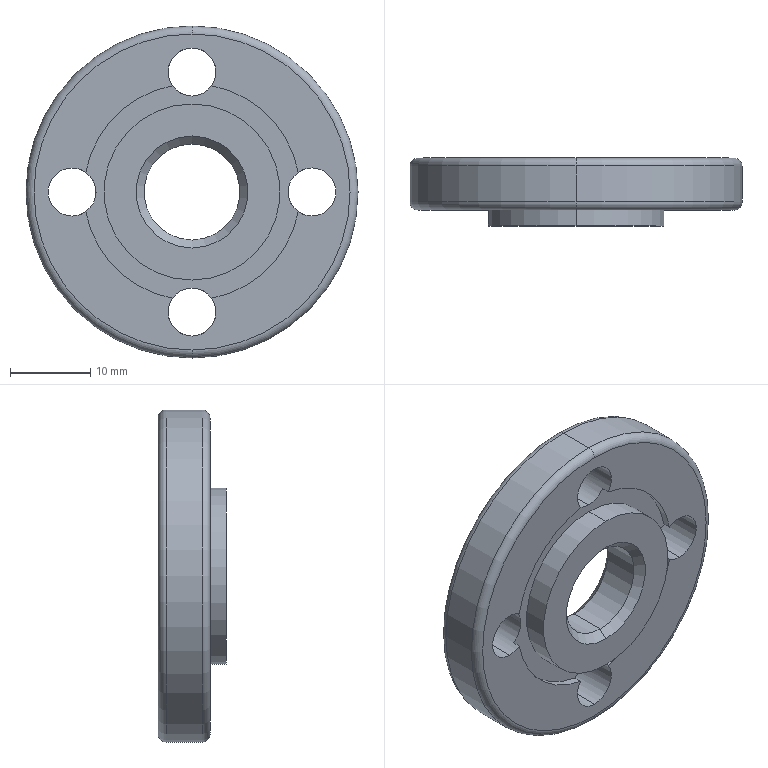Part | SolidWorks | features BaseBody 1 | 1 solid | 33 faces | box 41.5 x 8.5 x 41.5 mm | volume 6920 mm3 | cylinder 18 | cone 6 | plane 5 | torus 4 | commonest cylinder face diameters 6 x8 27 x4 12 x2 22 x2 41.5 x2
STEP:
#1=CARTESIAN_POINT('',(-15.,2.,3.));
#2=VERTEX_POINT('',#1);
#3=CARTESIAN_POINT('',(-15.,2.,-3.));
#4=VERTEX_POINT('',#3);
#5=CARTESIAN_POINT('',(-15.,2.,0.));
#6=DIRECTION('',(0.,-1.,0.));
#7=DIRECTION('',(0.,0.,-1.));
#8=AXIS2_PLACEMENT_3D('',#5,#6,#7);
#9=CIRCLE('',#8,3.);
#10=EDGE_CURVE('',#2,#4,#9,.T.);
#11=ORIENTED_EDGE('',*,*,#10,.T.);
#12=CARTESIAN_POINT('',(-15.,8.5,-3.));
#13=VERTEX_POINT('',#12);
#14=CARTESIAN_POINT('',(-15.,-1.5,-3.));
#15=DIRECTION('',(0.,1.,0.));
#16=VECTOR('',#15,1000.);
#17=LINE('',#14,#16);
#18=EDGE_CURVE('',#4,#13,#17,.T.);
#19=ORIENTED_EDGE('',*,*,#18,.T.);
#20=CARTESIAN_POINT('',(-15.,8.5,3.));
#21=VERTEX_POINT('',#20);
#22=CARTESIAN_POINT('',(-15.,8.5,0.));
#23=DIRECTION('',(0.,1.,0.));
#24=DIRECTION('',(1.,0.,0.));
#25=AXIS2_PLACEMENT_3D('',#22,#23,#24);
#26=CIRCLE('',#25,3.);
#27=EDGE_CURVE('',#13,#21,#26,.T.);
#28=ORIENTED_EDGE('',*,*,#27,.T.);
#29=CARTESIAN_POINT('',(-15.,-1.5,3.));
#30=DIRECTION('',(0.,1.,0.));
#31=VECTOR('',#30,1000.);
#32=LINE('',#29,#31);
#33=EDGE_CURVE('',#2,#21,#32,.T.);
#34=ORIENTED_EDGE('',*,*,#33,.F.);
#35=EDGE_LOOP('',(#11,#19,#28,#34));
#36=FACE_OUTER_BOUND('',#35,.T.);
#37=CARTESIAN_POINT('',(-15.,-1.5,0.));
#38=DIRECTION('',(0.,1.,0.));
#39=DIRECTION('',(0.,0.,1.));
#40=AXIS2_PLACEMENT_3D('',#37,#38,#39);
#41=CYLINDRICAL_SURFACE('',#40,3.);
#42=ADVANCED_FACE('',(#36),#41,.F.);
#43=CARTESIAN_POINT('',(-2.454,3.,13.275));
#44=VERTEX_POINT('',#43);
#45=CARTESIAN_POINT('',(0.,3.,12.));
#46=VERTEX_POINT('',#45);
#47=CARTESIAN_POINT('',(0.,3.,15.));
#48=DIRECTION('',(0.,-1.,0.));
#49=DIRECTION('',(0.,0.,-1.));
#50=AXIS2_PLACEMENT_3D('',#47,#48,#49);
#51=CIRCLE('',#50,3.);
#52=EDGE_CURVE('',#44,#46,#51,.T.);
#53=ORIENTED_EDGE('',*,*,#52,.T.);
#54=CARTESIAN_POINT('',(0.,7.35,12.));
#55=VERTEX_POINT('',#54);
#56=CARTESIAN_POINT('',(0.,-1.5,12.));
#57=DIRECTION('',(0.,1.,0.));
#58=VECTOR('',#57,1000.);
#59=LINE('',#56,#58);
#60=EDGE_CURVE('',#46,#55,#59,.T.);
#61=ORIENTED_EDGE('',*,*,#60,.T.);
#62=CARTESIAN_POINT('',(-2.203,8.5,12.964));
#63=VERTEX_POINT('',#62);
#64=CARTESIAN_POINT('',(0.,7.35,12.));
#65=CARTESIAN_POINT('',(-0.2354,7.35,12.));
#66=CARTESIAN_POINT('',(-0.4621,7.384,12.027));
#67=CARTESIAN_POINT('',(-0.9003,7.511,12.129));
#68=CARTESIAN_POINT('',(-1.104,7.601,12.203));
#69=CARTESIAN_POINT('',(-1.477,7.817,12.381));
#70=CARTESIAN_POINT('',(-1.646,7.942,12.485));
#71=CARTESIAN_POINT('',(-1.947,8.208,12.71));
#72=CARTESIAN_POINT('',(-2.082,8.35,12.833));
#73=CARTESIAN_POINT('',(-2.203,8.5,12.964));
#74=B_SPLINE_CURVE_WITH_KNOTS('',3,(#64,#65,#66,#67,#68,#69,#70,#71,#72,#73),.UNSPECIFIED.,.F.,.F.,(4,2,2,2,4),(0.,0.0006925,0.001385,0.002078,0.00277),.UNSPECIFIED.);
#75=EDGE_CURVE('',#55,#63,#74,.T.);
#76=ORIENTED_EDGE('',*,*,#75,.T.);
#77=CARTESIAN_POINT('',(0.,8.5,18.));
#78=VERTEX_POINT('',#77);
#79=CARTESIAN_POINT('',(0.,8.5,15.));
#80=DIRECTION('',(0.,1.,0.));
#81=DIRECTION('',(0.,0.,-1.));
#82=AXIS2_PLACEMENT_3D('',#79,#80,#81);
#83=CIRCLE('',#82,3.);
#84=EDGE_CURVE('',#63,#78,#83,.T.);
#85=ORIENTED_EDGE('',*,*,#84,.T.);
#86=CARTESIAN_POINT('',(0.,2.,18.));
#87=VERTEX_POINT('',#86);
#88=CARTESIAN_POINT('',(0.,-1.5,18.));
#89=DIRECTION('',(0.,1.,0.));
#90=VECTOR('',#89,1000.);
#91=LINE('',#88,#90);
#92=EDGE_CURVE('',#87,#78,#91,.T.);
#93=ORIENTED_EDGE('',*,*,#92,.F.);
#94=CARTESIAN_POINT('',(-2.454,2.,13.275));
#95=VERTEX_POINT('',#94);
#96=CARTESIAN_POINT('',(0.,2.,15.));
#97=DIRECTION('',(0.,-1.,0.));
#98=DIRECTION('',(0.,0.,-1.));
#99=AXIS2_PLACEMENT_3D('',#96,#97,#98);
#100=CIRCLE('',#99,3.);
#101=EDGE_CURVE('',#87,#95,#100,.T.);
#102=ORIENTED_EDGE('',*,*,#101,.T.);
#103=CARTESIAN_POINT('',(-2.454,3.5,13.275));
#104=DIRECTION('',(0.,1.,0.));
#105=VECTOR('',#104,1000.);
#106=LINE('',#103,#105);
#107=EDGE_CURVE('',#95,#44,#106,.T.);
#108=ORIENTED_EDGE('',*,*,#107,.T.);
#109=EDGE_LOOP('',(#53,#61,#76,#85,#93,#102,#108));
#110=FACE_OUTER_BOUND('',#109,.T.);
#111=CARTESIAN_POINT('',(0.,-1.5,15.));
#112=DIRECTION('',(0.,1.,0.));
#113=DIRECTION('',(0.,0.,1.));
#114=AXIS2_PLACEMENT_3D('',#111,#112,#113);
#115=CYLINDRICAL_SURFACE('',#114,3.);
#116=ADVANCED_FACE('',(#110),#115,.F.);
#117=CARTESIAN_POINT('',(13.275,2.,-2.454));
#118=VERTEX_POINT('',#117);
#119=CARTESIAN_POINT('',(15.,2.,-3.));
#120=VERTEX_POINT('',#119);
#121=CARTESIAN_POINT('',(15.,2.,0.));
#122=DIRECTION('',(0.,-1.,0.));
#123=DIRECTION('',(0.,0.,-1.));
#124=AXIS2_PLACEMENT_3D('',#121,#122,#123);
#125=CIRCLE('',#124,3.);
#126=EDGE_CURVE('',#118,#120,#125,.T.);
#127=ORIENTED_EDGE('',*,*,#126,.T.);
#128=CARTESIAN_POINT('',(15.,8.5,-3.));
#129=VERTEX_POINT('',#128);
#130=CARTESIAN_POINT('',(15.,-1.5,-3.));
#131=DIRECTION('',(0.,1.,0.));
#132=VECTOR('',#131,1000.);
#133=LINE('',#130,#132);
#134=EDGE_CURVE('',#120,#129,#133,.T.);
#135=ORIENTED_EDGE('',*,*,#134,.T.);
#136=CARTESIAN_POINT('',(12.964,8.5,-2.203));
#137=VERTEX_POINT('',#136);
#138=CARTESIAN_POINT('',(15.,8.5,0.));
#139=DIRECTION('',(0.,1.,0.));
#140=DIRECTION('',(-1.,0.,0.));
#141=AXIS2_PLACEMENT_3D('',#138,#139,#140);
#142=CIRCLE('',#141,3.);
#143=EDGE_CURVE('',#129,#137,#142,.T.);
#144=ORIENTED_EDGE('',*,*,#143,.T.);
#145=CARTESIAN_POINT('',(12.964,8.5,2.203));
#146=VERTEX_POINT('',#145);
#147=CARTESIAN_POINT('',(12.964,8.5,-2.203));
#148=CARTESIAN_POINT('',(12.833,8.35,-2.082));
#149=CARTESIAN_POINT('',(12.71,8.208,-1.948));
#150=CARTESIAN_POINT('',(12.485,7.942,-1.646));
#151=CARTESIAN_POINT('',(12.38,7.817,-1.477));
#152=CARTESIAN_POINT('',(12.203,7.602,-1.105));
#153=CARTESIAN_POINT('',(12.13,7.512,-0.9023));
#154=CARTESIAN_POINT('',(12.053,7.417,-0.5748));
#155=CARTESIAN_POINT('',(12.034,7.392,-0.4634));
#156=CARTESIAN_POINT('',(12.007,7.359,-0.2357));
#157=CARTESIAN_POINT('',(12.,7.35,-0.1181));
#158=CARTESIAN_POINT('',(12.,7.35,0.1144));
#159=CARTESIAN_POINT('',(12.007,7.358,0.2295));
#160=CARTESIAN_POINT('',(12.033,7.391,0.4574));
#161=CARTESIAN_POINT('',(12.053,7.416,0.5711));
#162=CARTESIAN_POINT('',(12.129,7.51,0.8984));
#163=CARTESIAN_POINT('',(12.203,7.601,1.103));
#164=CARTESIAN_POINT('',(12.468,7.923,1.66));
#165=CARTESIAN_POINT('',(12.701,8.2,1.961));
#166=CARTESIAN_POINT('',(12.964,8.5,2.203));
#167=B_SPLINE_CURVE_WITH_KNOTS('',3,(#147,#148,#149,#150,#151,#152,#153,#154,#155,#156,#157,#158,#159,#160,#161,#162,#163,#164,#165,#166),.UNSPECIFIED.,.F.,.F.,(4,2,2,2,2,2,2,2,2,4),(0.,0.0006916,0.001383,0.002075,0.00242,0.002766,0.003112,0.003458,0.004149,0.005533),.UNSPECIFIED.);
#168=EDGE_CURVE('',#137,#146,#167,.T.);
#169=ORIENTED_EDGE('',*,*,#168,.T.);
#170=CARTESIAN_POINT('',(15.,8.5,3.));
#171=VERTEX_POINT('',#170);
#172=CARTESIAN_POINT('',(15.,8.5,0.));
#173=DIRECTION('',(0.,1.,0.));
#174=DIRECTION('',(-1.,0.,0.));
#175=AXIS2_PLACEMENT_3D('',#172,#173,#174);
#176=CIRCLE('',#175,3.);
#177=EDGE_CURVE('',#146,#171,#176,.T.);
#178=ORIENTED_EDGE('',*,*,#177,.T.);
#179=CARTESIAN_POINT('',(15.,2.,3.));
#180=VERTEX_POINT('',#179);
#181=CARTESIAN_POINT('',(15.,-1.5,3.));
#182=DIRECTION('',(0.,1.,0.));
#183=VECTOR('',#182,1000.);
#184=LINE('',#181,#183);
#185=EDGE_CURVE('',#180,#171,#184,.T.);
#186=ORIENTED_EDGE('',*,*,#185,.F.);
#187=CARTESIAN_POINT('',(13.275,2.,2.454));
#188=VERTEX_POINT('',#187);
#189=CARTESIAN_POINT('',(15.,2.,0.));
#190=DIRECTION('',(0.,-1.,0.));
#191=DIRECTION('',(0.,0.,-1.));
#192=AXIS2_PLACEMENT_3D('',#189,#190,#191);
#193=CIRCLE('',#192,3.);
#194=EDGE_CURVE('',#180,#188,#193,.T.);
#195=ORIENTED_EDGE('',*,*,#194,.T.);
#196=CARTESIAN_POINT('',(13.275,3.,2.454));
#197=VERTEX_POINT('',#196);
#198=CARTESIAN_POINT('',(13.275,3.5,2.454));
#199=DIRECTION('',(0.,1.,0.));
#200=VECTOR('',#199,1000.);
#201=LINE('',#198,#200);
#202=EDGE_CURVE('',#188,#197,#201,.T.);
#203=ORIENTED_EDGE('',*,*,#202,.T.);
#204=CARTESIAN_POINT('',(13.275,3.,-2.454));
#205=VERTEX_POINT('',#204);
#206=CARTESIAN_POINT('',(15.,3.,0.));
#207=DIRECTION('',(0.,-1.,0.));
#208=DIRECTION('',(0.,0.,-1.));
#209=AXIS2_PLACEMENT_3D('',#206,#207,#208);
#210=CIRCLE('',#209,3.);
#211=EDGE_CURVE('',#197,#205,#210,.T.);
#212=ORIENTED_EDGE('',*,*,#211,.T.);
#213=CARTESIAN_POINT('',(13.275,3.5,-2.454));
#214=DIRECTION('',(0.,-1.,0.));
#215=VECTOR('',#214,1000.);
#216=LINE('',#213,#215);
#217=EDGE_CURVE('',#205,#118,#216,.T.);
#218=ORIENTED_EDGE('',*,*,#217,.T.);
#219=EDGE_LOOP('',(#127,#135,#144,#169,#178,#186,#195,#203,#212,#218));
#220=FACE_OUTER_BOUND('',#219,.T.);
#221=CARTESIAN_POINT('',(15.,-1.5,0.));
#222=DIRECTION('',(0.,1.,0.));
#223=DIRECTION('',(0.,0.,1.));
#224=AXIS2_PLACEMENT_3D('',#221,#222,#223);
#225=CYLINDRICAL_SURFACE('',#224,3.);
#226=ADVANCED_FACE('',(#220),#225,.F.);
#227=CARTESIAN_POINT('',(-2.454,2.,-13.275));
#228=VERTEX_POINT('',#227);
#229=CARTESIAN_POINT('',(0.,2.,-18.));
#230=VERTEX_POINT('',#229);
#231=CARTESIAN_POINT('',(0.,2.,-15.));
#232=DIRECTION('',(0.,-1.,0.));
#233=DIRECTION('',(0.,0.,-1.));
#234=AXIS2_PLACEMENT_3D('',#231,#232,#233);
#235=CIRCLE('',#234,3.);
#236=EDGE_CURVE('',#228,#230,#235,.T.);
#237=ORIENTED_EDGE('',*,*,#236,.T.);
#238=CARTESIAN_POINT('',(0.,8.5,-18.));
#239=VERTEX_POINT('',#238);
#240=CARTESIAN_POINT('',(0.,-1.5,-18.));
#241=DIRECTION('',(0.,1.,0.));
#242=VECTOR('',#241,1000.);
#243=LINE('',#240,#242);
#244=EDGE_CURVE('',#230,#239,#243,.T.);
#245=ORIENTED_EDGE('',*,*,#244,.T.);
#246=CARTESIAN_POINT('',(-2.203,8.5,-12.964));
#247=VERTEX_POINT('',#246);
#248=CARTESIAN_POINT('',(0.,8.5,-15.));
#249=DIRECTION('',(0.,1.,0.));
#250=DIRECTION('',(0.,0.,1.));
#251=AXIS2_PLACEMENT_3D('',#248,#249,#250);
#252=CIRCLE('',#251,3.);
#253=EDGE_CURVE('',#239,#247,#252,.T.);
#254=ORIENTED_EDGE('',*,*,#253,.T.);
#255=CARTESIAN_POINT('',(0.,7.35,-12.));
#256=VERTEX_POINT('',#255);
#257=CARTESIAN_POINT('',(-2.203,8.5,-12.964));
#258=CARTESIAN_POINT('',(-2.082,8.35,-12.833));
#259=CARTESIAN_POINT('',(-1.947,8.208,-12.71));
#260=CARTESIAN_POINT('',(-1.646,7.942,-12.485));
#261=CARTESIAN_POINT('',(-1.476,7.817,-12.38));
#262=CARTESIAN_POINT('',(-1.105,7.602,-12.203));
#263=CARTESIAN_POINT('',(-0.9015,7.511,-12.13));
#264=CARTESIAN_POINT('',(-0.4646,7.385,-12.028));
#265=CARTESIAN_POINT('',(-0.2349,7.35,-12.));
#266=CARTESIAN_POINT('',(0.,7.35,-12.));
#267=B_SPLINE_CURVE_WITH_KNOTS('',3,(#257,#258,#259,#260,#261,#262,#263,#264,#265,#266),.UNSPECIFIED.,.F.,.F.,(4,2,2,2,4),(0.,0.0006919,0.001384,0.002076,0.002768),.UNSPECIFIED.);
#268=EDGE_CURVE('',#247,#256,#267,.T.);
#269=ORIENTED_EDGE('',*,*,#268,.T.);
#270=CARTESIAN_POINT('',(0.,3.,-12.));
#271=VERTEX_POINT('',#270);
#272=CARTESIAN_POINT('',(0.,-1.5,-12.));
#273=DIRECTION('',(0.,1.,0.));
#274=VECTOR('',#273,1000.);
#275=LINE('',#272,#274);
#276=EDGE_CURVE('',#271,#256,#275,.T.);
#277=ORIENTED_EDGE('',*,*,#276,.F.);
#278=CARTESIAN_POINT('',(-2.454,3.,-13.275));
#279=VERTEX_POINT('',#278);
#280=CARTESIAN_POINT('',(0.,3.,-15.));
#281=DIRECTION('',(0.,-1.,0.));
#282=DIRECTION('',(0.,0.,-1.));
#283=AXIS2_PLACEMENT_3D('',#280,#281,#282);
#284=CIRCLE('',#283,3.);
#285=EDGE_CURVE('',#271,#279,#284,.T.);
#286=ORIENTED_EDGE('',*,*,#285,.T.);
#287=CARTESIAN_POINT('',(-2.454,3.5,-13.275));
#288=DIRECTION('',(0.,-1.,0.));
#289=VECTOR('',#288,1000.);
#290=LINE('',#287,#289);
#291=EDGE_CURVE('',#279,#228,#290,.T.);
#292=ORIENTED_EDGE('',*,*,#291,.T.);
#293=EDGE_LOOP('',(#237,#245,#254,#269,#277,#286,#292));
#294=FACE_OUTER_BOUND('',#293,.T.);
#295=CARTESIAN_POINT('',(0.,-1.5,-15.));
#296=DIRECTION('',(0.,1.,0.));
#297=DIRECTION('',(0.,0.,1.));
#298=AXIS2_PLACEMENT_3D('',#295,#296,#297);
#299=CYLINDRICAL_SURFACE('',#298,3.);
#300=ADVANCED_FACE('',(#294),#299,.F.);
#301=CARTESIAN_POINT('',(0.,6.6,11.25));
#302=VERTEX_POINT('',#301);
#303=CARTESIAN_POINT('',(0.,6.6,-11.25));
#304=VERTEX_POINT('',#303);
#305=CARTESIAN_POINT('',(0.,6.6,0.));
#306=DIRECTION('',(0.,-1.,0.));
#307=DIRECTION('',(0.,0.,-1.));
#308=AXIS2_PLACEMENT_3D('',#305,#306,#307);
#309=CIRCLE('',#308,11.25);
#310=EDGE_CURVE('',#302,#304,#309,.T.);
#311=ORIENTED_EDGE('',*,*,#310,.T.);
#312=CARTESIAN_POINT('',(0.,8.5,-13.15));
#313=DIRECTION('',(0.,0.7071,-0.7071));
#314=VECTOR('',#313,1000.);
#315=LINE('',#312,#314);
#316=EDGE_CURVE('',#304,#256,#315,.T.);
#317=ORIENTED_EDGE('',*,*,#316,.T.);
#318=ORIENTED_EDGE('',*,*,#268,.F.);
#319=CARTESIAN_POINT('',(-12.964,8.5,-2.203));
#320=VERTEX_POINT('',#319);
#321=CARTESIAN_POINT('',(0.,8.5,0.));
#322=DIRECTION('',(0.,-1.,0.));
#323=DIRECTION('',(0.,0.,1.));
#324=AXIS2_PLACEMENT_3D('',#321,#322,#323);
#325=CIRCLE('',#324,13.15);
#326=EDGE_CURVE('',#320,#247,#325,.T.);
#327=ORIENTED_EDGE('',*,*,#326,.F.);
#328=CARTESIAN_POINT('',(-12.964,8.5,2.203));
#329=VERTEX_POINT('',#328);
#330=CARTESIAN_POINT('',(-12.964,8.5,2.203));
#331=CARTESIAN_POINT('',(-12.833,8.35,2.082));
#332=CARTESIAN_POINT('',(-12.71,8.208,1.948));
#333=CARTESIAN_POINT('',(-12.485,7.942,1.646));
#334=CARTESIAN_POINT('',(-12.38,7.817,1.477));
#335=CARTESIAN_POINT('',(-12.203,7.602,1.105));
#336=CARTESIAN_POINT('',(-12.13,7.512,0.9023));
#337=CARTESIAN_POINT('',(-12.053,7.417,0.5748));
#338=CARTESIAN_POINT('',(-12.034,7.392,0.4634));
#339=CARTESIAN_POINT('',(-12.007,7.359,0.2357));
#340=CARTESIAN_POINT('',(-12.,7.35,0.1181));
#341=CARTESIAN_POINT('',(-12.,7.35,-0.1144));
#342=CARTESIAN_POINT('',(-12.007,7.358,-0.2295));
#343=CARTESIAN_POINT('',(-12.033,7.391,-0.4574));
#344=CARTESIAN_POINT('',(-12.053,7.416,-0.5711));
#345=CARTESIAN_POINT('',(-12.129,7.51,-0.8984));
#346=CARTESIAN_POINT('',(-12.203,7.601,-1.103));
#347=CARTESIAN_POINT('',(-12.468,7.923,-1.66));
#348=CARTESIAN_POINT('',(-12.701,8.2,-1.961));
#349=CARTESIAN_POINT('',(-12.964,8.5,-2.203));
#350=B_SPLINE_CURVE_WITH_KNOTS('',3,(#330,#331,#332,#333,#334,#335,#336,#337,#338,#339,#340,#341,#342,#343,#344,#345,#346,#347,#348,#349),.UNSPECIFIED.,.F.,.F.,(4,2,2,2,2,2,2,2,2,4),(0.,0.0006916,0.001383,0.002075,0.00242,0.002766,0.003112,0.003458,0.004149,0.005533),.UNSPECIFIED.);
#351=EDGE_CURVE('',#329,#320,#350,.T.);
#352=ORIENTED_EDGE('',*,*,#351,.F.);
#353=CARTESIAN_POINT('',(0.,8.5,0.));
#354=DIRECTION('',(0.,-1.,0.));
#355=DIRECTION('',(0.,0.,1.));
#356=AXIS2_PLACEMENT_3D('',#353,#354,#355);
#357=CIRCLE('',#356,13.15);
#358=EDGE_CURVE('',#63,#329,#357,.T.);
#359=ORIENTED_EDGE('',*,*,#358,.F.);
#360=ORIENTED_EDGE('',*,*,#75,.F.);
#361=CARTESIAN_POINT('',(0.,8.5,13.15));
#362=DIRECTION('',(0.,0.7071,0.7071));
#363=VECTOR('',#362,1000.);
#364=LINE('',#361,#363);
#365=EDGE_CURVE('',#302,#55,#364,.T.);
#366=ORIENTED_EDGE('',*,*,#365,.F.);
#367=EDGE_LOOP('',(#311,#317,#318,#327,#352,#359,#360,#366));
#368=FACE_OUTER_BOUND('',#367,.T.);
#369=CARTESIAN_POINT('',(0.,8.5,0.));
#370=DIRECTION('',(0.,1.,0.));
#371=DIRECTION('',(0.,0.,1.));
#372=AXIS2_PLACEMENT_3D('',#369,#370,#371);
#373=CONICAL_SURFACE('',#372,13.15,0.7854);
#374=ADVANCED_FACE('',(#368),#373,.F.);
#375=CARTESIAN_POINT('',(0.,7.5,-20.75));
#376=VERTEX_POINT('',#375);
#377=CARTESIAN_POINT('',(0.,7.5,20.75));
#378=VERTEX_POINT('',#377);
#379=CARTESIAN_POINT('',(0.,7.5,0.));
#380=DIRECTION('',(0.,-1.,0.));
#381=DIRECTION('',(0.,0.,1.));
#382=AXIS2_PLACEMENT_3D('',#379,#380,#381);
#383=CIRCLE('',#382,20.75);
#384=EDGE_CURVE('',#376,#378,#383,.T.);
#385=ORIENTED_EDGE('',*,*,#384,.F.);
#386=CARTESIAN_POINT('',(0.,8.5,-19.75));
#387=VERTEX_POINT('',#386);
#388=CARTESIAN_POINT('',(0.,7.5,-19.75));
#389=DIRECTION('',(1.,0.,0.));
#390=DIRECTION('',(0.,0.,-1.));
#391=AXIS2_PLACEMENT_3D('',#388,#389,#390);
#392=CIRCLE('',#391,1.);
#393=EDGE_CURVE('',#376,#387,#392,.T.);
#394=ORIENTED_EDGE('',*,*,#393,.T.);
#395=CARTESIAN_POINT('',(0.,8.5,19.75));
#396=VERTEX_POINT('',#395);
#397=CARTESIAN_POINT('',(0.,8.5,0.));
#398=DIRECTION('',(0.,1.,0.));
#399=DIRECTION('',(0.,0.,1.));
#400=AXIS2_PLACEMENT_3D('',#397,#398,#399);
#401=CIRCLE('',#400,19.75);
#402=EDGE_CURVE('',#396,#387,#401,.T.);
#403=ORIENTED_EDGE('',*,*,#402,.F.);
#404=CARTESIAN_POINT('',(0.,7.5,19.75));
#405=DIRECTION('',(-1.,0.,0.));
#406=DIRECTION('',(0.,0.,1.));
#407=AXIS2_PLACEMENT_3D('',#404,#405,#406);
#408=CIRCLE('',#407,1.);
#409=EDGE_CURVE('',#378,#396,#408,.T.);
#410=ORIENTED_EDGE('',*,*,#409,.F.);
#411=EDGE_LOOP('',(#385,#394,#403,#410));
#412=FACE_OUTER_BOUND('',#411,.T.);
#413=CARTESIAN_POINT('',(0.,7.5,0.));
#414=DIRECTION('',(0.,1.,0.));
#415=DIRECTION('',(0.,0.,1.));
#416=AXIS2_PLACEMENT_3D('',#413,#414,#415);
#417=TOROIDAL_SURFACE('',#416,19.75,1.);
#418=ADVANCED_FACE('',(#412),#417,.T.);
#419=CARTESIAN_POINT('',(0.,3.,20.75));
#420=VERTEX_POINT('',#419);
#421=CARTESIAN_POINT('',(0.,3.,-20.75));
#422=VERTEX_POINT('',#421);
#423=CARTESIAN_POINT('',(0.,3.,0.));
#424=DIRECTION('',(0.,1.,0.));
#425=DIRECTION('',(0.,0.,-1.));
#426=AXIS2_PLACEMENT_3D('',#423,#424,#425);
#427=CIRCLE('',#426,20.75);
#428=EDGE_CURVE('',#420,#422,#427,.T.);
#429=ORIENTED_EDGE('',*,*,#428,.F.);
#430=CARTESIAN_POINT('',(0.,2.,19.75));
#431=VERTEX_POINT('',#430);
#432=CARTESIAN_POINT('',(0.,3.,19.75));
#433=DIRECTION('',(1.,0.,0.));
#434=DIRECTION('',(0.,0.,-1.));
#435=AXIS2_PLACEMENT_3D('',#432,#433,#434);
#436=CIRCLE('',#435,1.);
#437=EDGE_CURVE('',#420,#431,#436,.T.);
#438=ORIENTED_EDGE('',*,*,#437,.T.);
#439=CARTESIAN_POINT('',(0.,2.,-19.75));
#440=VERTEX_POINT('',#439);
#441=CARTESIAN_POINT('',(0.,2.,0.));
#442=DIRECTION('',(0.,-1.,0.));
#443=DIRECTION('',(0.,0.,-1.));
#444=AXIS2_PLACEMENT_3D('',#441,#442,#443);
#445=CIRCLE('',#444,19.75);
#446=EDGE_CURVE('',#440,#431,#445,.T.);
#447=ORIENTED_EDGE('',*,*,#446,.F.);
#448=CARTESIAN_POINT('',(0.,3.,-19.75));
#449=DIRECTION('',(-1.,0.,0.));
#450=DIRECTION('',(0.,0.,1.));
#451=AXIS2_PLACEMENT_3D('',#448,#449,#450);
#452=CIRCLE('',#451,1.);
#453=EDGE_CURVE('',#422,#440,#452,.T.);
#454=ORIENTED_EDGE('',*,*,#453,.F.);
#455=EDGE_LOOP('',(#429,#438,#447,#454));
#456=FACE_OUTER_BOUND('',#455,.T.);
#457=CARTESIAN_POINT('',(0.,3.,0.));
#458=DIRECTION('',(0.,-1.,0.));
#459=DIRECTION('',(0.,0.,-1.));
#460=AXIS2_PLACEMENT_3D('',#457,#458,#459);
#461=TOROIDAL_SURFACE('',#460,19.75,1.);
#462=ADVANCED_FACE('',(#456),#461,.T.);
#463=CARTESIAN_POINT('',(0.,1.,6.));
#464=VERTEX_POINT('',#463);
#465=CARTESIAN_POINT('',(0.,1.,-6.));
#466=VERTEX_POINT('',#465);
#467=CARTESIAN_POINT('',(0.,1.,0.));
#468=DIRECTION('',(0.,-1.,0.));
#469=DIRECTION('',(0.,0.,-1.));
#470=AXIS2_PLACEMENT_3D('',#467,#468,#469);
#471=CIRCLE('',#470,6.);
#472=EDGE_CURVE('',#464,#466,#471,.T.);
#473=ORIENTED_EDGE('',*,*,#472,.F.);
#474=CARTESIAN_POINT('',(0.,0.,7.));
#475=VERTEX_POINT('',#474);
#476=CARTESIAN_POINT('',(0.,1.,6.));
#477=DIRECTION('',(0.,-0.7071,0.7071));
#478=VECTOR('',#477,1000.);
#479=LINE('',#476,#478);
#480=EDGE_CURVE('',#464,#475,#479,.T.);
#481=ORIENTED_EDGE('',*,*,#480,.T.);
#482=CARTESIAN_POINT('',(0.,0.,-7.));
#483=VERTEX_POINT('',#482);
#484=CARTESIAN_POINT('',(0.,0.,0.));
#485=DIRECTION('',(0.,1.,0.));
#486=DIRECTION('',(0.,0.,-1.));
#487=AXIS2_PLACEMENT_3D('',#484,#485,#486);
#488=CIRCLE('',#487,7.);
#489=EDGE_CURVE('',#483,#475,#488,.T.);
#490=ORIENTED_EDGE('',*,*,#489,.F.);
#491=CARTESIAN_POINT('',(0.,1.,-6.));
#492=DIRECTION('',(0.,-0.7071,-0.7071));
#493=VECTOR('',#492,1000.);
#494=LINE('',#491,#493);
#495=EDGE_CURVE('',#466,#483,#494,.T.);
#496=ORIENTED_EDGE('',*,*,#495,.F.);
#497=EDGE_LOOP('',(#473,#481,#490,#496));
#498=FACE_OUTER_BOUND('',#497,.T.);
#499=CARTESIAN_POINT('',(0.,1.,0.));
#500=DIRECTION('',(0.,-1.,0.));
#501=DIRECTION('',(0.,0.,-1.));
#502=AXIS2_PLACEMENT_3D('',#499,#500,#501);
#503=CONICAL_SURFACE('',#502,6.,0.7854);
#504=ADVANCED_FACE('',(#498),#503,.F.);
#505=CARTESIAN_POINT('',(0.,5.6,-6.));
#506=VERTEX_POINT('',#505);
#507=CARTESIAN_POINT('',(0.,5.6,6.));
#508=VERTEX_POINT('',#507);
#509=CARTESIAN_POINT('',(0.,5.6,0.));
#510=DIRECTION('',(0.,1.,0.));
#511=DIRECTION('',(0.,0.,1.));
#512=AXIS2_PLACEMENT_3D('',#509,#510,#511);
#513=CIRCLE('',#512,6.);
#514=EDGE_CURVE('',#506,#508,#513,.T.);
#515=ORIENTED_EDGE('',*,*,#514,.F.);
#516=CARTESIAN_POINT('',(0.,6.6,-7.));
#517=VERTEX_POINT('',#516);
#518=CARTESIAN_POINT('',(0.,6.6,-7.));
#519=DIRECTION('',(0.,0.7071,-0.7071));
#520=VECTOR('',#519,1000.);
#521=LINE('',#518,#520);
#522=EDGE_CURVE('',#506,#517,#521,.T.);
#523=ORIENTED_EDGE('',*,*,#522,.T.);
#524=CARTESIAN_POINT('',(0.,6.6,7.));
#525=VERTEX_POINT('',#524);
#526=CARTESIAN_POINT('',(0.,6.6,0.));
#527=DIRECTION('',(0.,-1.,0.));
#528=DIRECTION('',(0.,0.,1.));
#529=AXIS2_PLACEMENT_3D('',#526,#527,#528);
#530=CIRCLE('',#529,7.);
#531=EDGE_CURVE('',#525,#517,#530,.T.);
#532=ORIENTED_EDGE('',*,*,#531,.F.);
#533=CARTESIAN_POINT('',(0.,6.6,7.));
#534=DIRECTION('',(0.,0.7071,0.7071));
#535=VECTOR('',#534,1000.);
#536=LINE('',#533,#535);
#537=EDGE_CURVE('',#508,#525,#536,.T.);
#538=ORIENTED_EDGE('',*,*,#537,.F.);
#539=EDGE_LOOP('',(#515,#523,#532,#538));
#540=FACE_OUTER_BOUND('',#539,.T.);
#541=CARTESIAN_POINT('',(0.,6.6,0.));
#542=DIRECTION('',(0.,1.,0.));
#543=DIRECTION('',(0.,0.,1.));
#544=AXIS2_PLACEMENT_3D('',#541,#542,#543);
#545=CONICAL_SURFACE('',#544,7.,0.7854);
#546=ADVANCED_FACE('',(#540),#545,.F.);
#547=ORIENTED_EDGE('',*,*,#384,.T.);
#548=CARTESIAN_POINT('',(0.,0.,20.75));
#549=DIRECTION('',(0.,-1.,0.));
#550=VECTOR('',#549,1000.);
#551=LINE('',#548,#550);
#552=EDGE_CURVE('',#378,#420,#551,.T.);
#553=ORIENTED_EDGE('',*,*,#552,.T.);
#554=ORIENTED_EDGE('',*,*,#428,.T.);
#555=CARTESIAN_POINT('',(0.,0.,-20.75));
#556=DIRECTION('',(0.,-1.,0.));
#557=VECTOR('',#556,1000.);
#558=LINE('',#555,#557);
#559=EDGE_CURVE('',#376,#422,#558,.T.);
#560=ORIENTED_EDGE('',*,*,#559,.F.);
#561=EDGE_LOOP('',(#547,#553,#554,#560));
#562=FACE_OUTER_BOUND('',#561,.T.);
#563=CARTESIAN_POINT('',(0.,0.,0.));
#564=DIRECTION('',(0.,-1.,0.));
#565=DIRECTION('',(0.,0.,-1.));
#566=AXIS2_PLACEMENT_3D('',#563,#564,#565);
#567=CYLINDRICAL_SURFACE('',#566,20.75);
#568=ADVANCED_FACE('',(#562),#567,.T.);
#569=CARTESIAN_POINT('',(0.,3.,-11.));
#570=VERTEX_POINT('',#569);
#571=CARTESIAN_POINT('',(0.,3.,11.));
#572=VERTEX_POINT('',#571);
#573=CARTESIAN_POINT('',(0.,3.,0.));
#574=DIRECTION('',(0.,-1.,0.));
#575=DIRECTION('',(0.,0.,-1.));
#576=AXIS2_PLACEMENT_3D('',#573,#574,#575);
#577=CIRCLE('',#576,11.);
#578=EDGE_CURVE('',#570,#572,#577,.T.);
#579=ORIENTED_EDGE('',*,*,#578,.T.);
#580=CARTESIAN_POINT('',(0.,0.,11.));
#581=VERTEX_POINT('',#580);
#582=CARTESIAN_POINT('',(0.,0.,11.));
#583=DIRECTION('',(0.,-1.,0.));
#584=VECTOR('',#583,1000.);
#585=LINE('',#582,#584);
#586=EDGE_CURVE('',#572,#581,#585,.T.);
#587=ORIENTED_EDGE('',*,*,#586,.T.);
#588=CARTESIAN_POINT('',(0.,0.,-11.));
#589=VERTEX_POINT('',#588);
#590=CARTESIAN_POINT('',(0.,0.,0.));
#591=DIRECTION('',(0.,-1.,0.));
#592=DIRECTION('',(0.,0.,-1.));
#593=AXIS2_PLACEMENT_3D('',#590,#591,#592);
#594=CIRCLE('',#593,11.);
#595=EDGE_CURVE('',#589,#581,#594,.T.);
#596=ORIENTED_EDGE('',*,*,#595,.F.);
#597=CARTESIAN_POINT('',(0.,0.,-11.));
#598=DIRECTION('',(0.,-1.,0.));
#599=VECTOR('',#598,1000.);
#600=LINE('',#597,#599);
#601=EDGE_CURVE('',#570,#589,#600,.T.);
#602=ORIENTED_EDGE('',*,*,#601,.F.);
#603=EDGE_LOOP('',(#579,#587,#596,#602));
#604=FACE_OUTER_BOUND('',#603,.T.);
#605=CARTESIAN_POINT('',(0.,0.,0.));
#606=DIRECTION('',(0.,-1.,0.));
#607=DIRECTION('',(0.,0.,-1.));
#608=AXIS2_PLACEMENT_3D('',#605,#606,#607);
#609=CYLINDRICAL_SURFACE('',#608,11.);
#610=ADVANCED_FACE('',(#604),#609,.T.);
#611=ORIENTED_EDGE('',*,*,#514,.T.);
#612=CARTESIAN_POINT('',(0.,0.,6.));
#613=DIRECTION('',(0.,-1.,0.));
#614=VECTOR('',#613,1000.);
#615=LINE('',#612,#614);
#616=EDGE_CURVE('',#508,#464,#615,.T.);
#617=ORIENTED_EDGE('',*,*,#616,.T.);
#618=ORIENTED_EDGE('',*,*,#472,.T.);
#619=CARTESIAN_POINT('',(0.,0.,-6.));
#620=DIRECTION('',(0.,-1.,0.));
#621=VECTOR('',#620,1000.);
#622=LINE('',#619,#621);
#623=EDGE_CURVE('',#506,#466,#622,.T.);
#624=ORIENTED_EDGE('',*,*,#623,.F.);
#625=EDGE_LOOP('',(#611,#617,#618,#624));
#626=FACE_OUTER_BOUND('',#625,.T.);
#627=CARTESIAN_POINT('',(0.,0.,0.));
#628=DIRECTION('',(0.,-1.,0.));
#629=DIRECTION('',(0.,0.,-1.));
#630=AXIS2_PLACEMENT_3D('',#627,#628,#629);
#631=CYLINDRICAL_SURFACE('',#630,6.);
#632=ADVANCED_FACE('',(#626),#631,.F.);
#633=ORIENTED_EDGE('',*,*,#531,.T.);
#634=CARTESIAN_POINT('',(0.,6.6,0.));
#635=DIRECTION('',(0.,-1.,0.));
#636=DIRECTION('',(0.,0.,1.));
#637=AXIS2_PLACEMENT_3D('',#634,#635,#636);
#638=CIRCLE('',#637,7.);
#639=EDGE_CURVE('',#517,#525,#638,.T.);
#640=ORIENTED_EDGE('',*,*,#639,.T.);
#641=EDGE_LOOP('',(#633,#640));
#642=FACE_BOUND('',#641,.T.);
#643=ORIENTED_EDGE('',*,*,#310,.F.);
#644=CARTESIAN_POINT('',(0.,6.6,0.));
#645=DIRECTION('',(0.,-1.,0.));
#646=DIRECTION('',(0.,0.,-1.));
#647=AXIS2_PLACEMENT_3D('',#644,#645,#646);
#648=CIRCLE('',#647,11.25);
#649=EDGE_CURVE('',#304,#302,#648,.T.);
#650=ORIENTED_EDGE('',*,*,#649,.F.);
#651=EDGE_LOOP('',(#643,#650));
#652=FACE_OUTER_BOUND('',#651,.T.);
#653=CARTESIAN_POINT('',(6.,6.6,0.));
#654=DIRECTION('',(0.,1.,0.));
#655=DIRECTION('',(1.,0.,0.));
#656=AXIS2_PLACEMENT_3D('',#653,#654,#655);
#657=PLANE('',#656);
#658=ADVANCED_FACE('',(#642,#652),#657,.T.);
#659=CARTESIAN_POINT('',(-15.,8.5,0.));
#660=DIRECTION('',(0.,1.,0.));
#661=DIRECTION('',(1.,0.,0.));
#662=AXIS2_PLACEMENT_3D('',#659,#660,#661);
#663=CIRCLE('',#662,3.);
#664=EDGE_CURVE('',#320,#13,#663,.T.);
#665=ORIENTED_EDGE('',*,*,#664,.F.);
#666=ORIENTED_EDGE('',*,*,#326,.T.);
#667=ORIENTED_EDGE('',*,*,#253,.F.);
#668=CARTESIAN_POINT('',(2.203,8.5,-12.964));
#669=VERTEX_POINT('',#668);
#670=CARTESIAN_POINT('',(0.,8.5,-15.));
#671=DIRECTION('',(0.,1.,0.));
#672=DIRECTION('',(0.,0.,1.));
#673=AXIS2_PLACEMENT_3D('',#670,#671,#672);
#674=CIRCLE('',#673,3.);
#675=EDGE_CURVE('',#669,#239,#674,.T.);
#676=ORIENTED_EDGE('',*,*,#675,.F.);
#677=CARTESIAN_POINT('',(0.,8.5,0.));
#678=DIRECTION('',(0.,-1.,0.));
#679=DIRECTION('',(0.,0.,1.));
#680=AXIS2_PLACEMENT_3D('',#677,#678,#679);
#681=CIRCLE('',#680,13.15);
#682=EDGE_CURVE('',#669,#137,#681,.T.);
#683=ORIENTED_EDGE('',*,*,#682,.T.);
#684=ORIENTED_EDGE('',*,*,#143,.F.);
#685=CARTESIAN_POINT('',(15.,8.5,0.));
#686=DIRECTION('',(0.,1.,0.));
#687=DIRECTION('',(-1.,0.,0.));
#688=AXIS2_PLACEMENT_3D('',#685,#686,#687);
#689=CIRCLE('',#688,3.);
#690=EDGE_CURVE('',#171,#129,#689,.T.);
#691=ORIENTED_EDGE('',*,*,#690,.F.);
#692=ORIENTED_EDGE('',*,*,#177,.F.);
#693=CARTESIAN_POINT('',(2.203,8.5,12.964));
#694=VERTEX_POINT('',#693);
#695=CARTESIAN_POINT('',(0.,8.5,0.));
#696=DIRECTION('',(0.,-1.,0.));
#697=DIRECTION('',(0.,0.,1.));
#698=AXIS2_PLACEMENT_3D('',#695,#696,#697);
#699=CIRCLE('',#698,13.15);
#700=EDGE_CURVE('',#146,#694,#699,.T.);
#701=ORIENTED_EDGE('',*,*,#700,.T.);
#702=CARTESIAN_POINT('',(0.,8.5,15.));
#703=DIRECTION('',(0.,1.,0.));
#704=DIRECTION('',(0.,0.,-1.));
#705=AXIS2_PLACEMENT_3D('',#702,#703,#704);
#706=CIRCLE('',#705,3.);
#707=EDGE_CURVE('',#78,#694,#706,.T.);
#708=ORIENTED_EDGE('',*,*,#707,.F.);
#709=ORIENTED_EDGE('',*,*,#84,.F.);
#710=ORIENTED_EDGE('',*,*,#358,.T.);
#711=CARTESIAN_POINT('',(-15.,8.5,0.));
#712=DIRECTION('',(0.,1.,0.));
#713=DIRECTION('',(1.,0.,0.));
#714=AXIS2_PLACEMENT_3D('',#711,#712,#713);
#715=CIRCLE('',#714,3.);
#716=EDGE_CURVE('',#21,#329,#715,.T.);
#717=ORIENTED_EDGE('',*,*,#716,.F.);
#718=ORIENTED_EDGE('',*,*,#27,.F.);
#719=EDGE_LOOP('',(#665,#666,#667,#676,#683,#684,#691,#692,#701,#708,#709,#710,#717,#718));
#720=FACE_BOUND('',#719,.T.);
#721=ORIENTED_EDGE('',*,*,#402,.T.);
#722=CARTESIAN_POINT('',(0.,8.5,0.));
#723=DIRECTION('',(0.,1.,0.));
#724=DIRECTION('',(0.,0.,1.));
#725=AXIS2_PLACEMENT_3D('',#722,#723,#724);
#726=CIRCLE('',#725,19.75);
#727=EDGE_CURVE('',#387,#396,#726,.T.);
#728=ORIENTED_EDGE('',*,*,#727,.T.);
#729=EDGE_LOOP('',(#721,#728));
#730=FACE_OUTER_BOUND('',#729,.T.);
#731=CARTESIAN_POINT('',(20.75,8.5,0.));
#732=DIRECTION('',(0.,1.,0.));
#733=DIRECTION('',(1.,0.,0.));
#734=AXIS2_PLACEMENT_3D('',#731,#732,#733);
#735=PLANE('',#734);
#736=ADVANCED_FACE('',(#720,#730),#735,.T.);
#737=CARTESIAN_POINT('',(-13.275,2.,2.454));
#738=VERTEX_POINT('',#737);
#739=CARTESIAN_POINT('',(-15.,2.,0.));
#740=DIRECTION('',(0.,-1.,0.));
#741=DIRECTION('',(0.,0.,-1.));
#742=AXIS2_PLACEMENT_3D('',#739,#740,#741);
#743=CIRCLE('',#742,3.);
#744=EDGE_CURVE('',#738,#2,#743,.T.);
#745=ORIENTED_EDGE('',*,*,#744,.F.);
#746=CARTESIAN_POINT('',(0.,2.,0.));
#747=DIRECTION('',(0.,-1.,0.));
#748=DIRECTION('',(0.,0.,-1.));
#749=AXIS2_PLACEMENT_3D('',#746,#747,#748);
#750=CIRCLE('',#749,13.5);
#751=EDGE_CURVE('',#95,#738,#750,.T.);
#752=ORIENTED_EDGE('',*,*,#751,.F.);
#753=ORIENTED_EDGE('',*,*,#101,.F.);
#754=CARTESIAN_POINT('',(2.454,2.,13.275));
#755=VERTEX_POINT('',#754);
#756=CARTESIAN_POINT('',(0.,2.,15.));
#757=DIRECTION('',(0.,-1.,0.));
#758=DIRECTION('',(0.,0.,-1.));
#759=AXIS2_PLACEMENT_3D('',#756,#757,#758);
#760=CIRCLE('',#759,3.);
#761=EDGE_CURVE('',#755,#87,#760,.T.);
#762=ORIENTED_EDGE('',*,*,#761,.F.);
#763=CARTESIAN_POINT('',(0.,2.,0.));
#764=DIRECTION('',(0.,-1.,0.));
#765=DIRECTION('',(0.,0.,-1.));
#766=AXIS2_PLACEMENT_3D('',#763,#764,#765);
#767=CIRCLE('',#766,13.5);
#768=EDGE_CURVE('',#188,#755,#767,.T.);
#769=ORIENTED_EDGE('',*,*,#768,.F.);
#770=ORIENTED_EDGE('',*,*,#194,.F.);
#771=CARTESIAN_POINT('',(15.,2.,0.));
#772=DIRECTION('',(0.,-1.,0.));
#773=DIRECTION('',(0.,0.,-1.));
#774=AXIS2_PLACEMENT_3D('',#771,#772,#773);
#775=CIRCLE('',#774,3.);
#776=EDGE_CURVE('',#120,#180,#775,.T.);
#777=ORIENTED_EDGE('',*,*,#776,.F.);
#778=ORIENTED_EDGE('',*,*,#126,.F.);
#779=CARTESIAN_POINT('',(2.454,2.,-13.275));
#780=VERTEX_POINT('',#779);
#781=CARTESIAN_POINT('',(0.,2.,0.));
#782=DIRECTION('',(0.,-1.,0.));
#783=DIRECTION('',(0.,0.,-1.));
#784=AXIS2_PLACEMENT_3D('',#781,#782,#783);
#785=CIRCLE('',#784,13.5);
#786=EDGE_CURVE('',#780,#118,#785,.T.);
#787=ORIENTED_EDGE('',*,*,#786,.F.);
#788=CARTESIAN_POINT('',(0.,2.,-15.));
#789=DIRECTION('',(0.,-1.,0.));
#790=DIRECTION('',(0.,0.,-1.));
#791=AXIS2_PLACEMENT_3D('',#788,#789,#790);
#792=CIRCLE('',#791,3.);
#793=EDGE_CURVE('',#230,#780,#792,.T.);
#794=ORIENTED_EDGE('',*,*,#793,.F.);
#795=ORIENTED_EDGE('',*,*,#236,.F.);
#796=CARTESIAN_POINT('',(-13.275,2.,-2.454));
#797=VERTEX_POINT('',#796);
#798=CARTESIAN_POINT('',(0.,2.,0.));
#799=DIRECTION('',(0.,-1.,0.));
#800=DIRECTION('',(0.,0.,-1.));
#801=AXIS2_PLACEMENT_3D('',#798,#799,#800);
#802=CIRCLE('',#801,13.5);
#803=EDGE_CURVE('',#797,#228,#802,.T.);
#804=ORIENTED_EDGE('',*,*,#803,.F.);
#805=CARTESIAN_POINT('',(-15.,2.,0.));
#806=DIRECTION('',(0.,-1.,0.));
#807=DIRECTION('',(0.,0.,-1.));
#808=AXIS2_PLACEMENT_3D('',#805,#806,#807);
#809=CIRCLE('',#808,3.);
#810=EDGE_CURVE('',#4,#797,#809,.T.);
#811=ORIENTED_EDGE('',*,*,#810,.F.);
#812=ORIENTED_EDGE('',*,*,#10,.F.);
#813=EDGE_LOOP('',(#745,#752,#753,#762,#769,#770,#777,#778,#787,#794,#795,#804,#811,#812));
#814=FACE_BOUND('',#813,.T.);
#815=ORIENTED_EDGE('',*,*,#446,.T.);
#816=CARTESIAN_POINT('',(0.,2.,0.));
#817=DIRECTION('',(0.,-1.,0.));
#818=DIRECTION('',(0.,0.,-1.));
#819=AXIS2_PLACEMENT_3D('',#816,#817,#818);
#820=CIRCLE('',#819,19.75);
#821=EDGE_CURVE('',#431,#440,#820,.T.);
#822=ORIENTED_EDGE('',*,*,#821,.T.);
#823=EDGE_LOOP('',(#815,#822));
#824=FACE_OUTER_BOUND('',#823,.T.);
#825=CARTESIAN_POINT('',(13.5,2.,0.));
#826=DIRECTION('',(0.,-1.,0.));
#827=DIRECTION('',(0.,0.,-1.));
#828=AXIS2_PLACEMENT_3D('',#825,#826,#827);
#829=PLANE('',#828);
#830=ADVANCED_FACE('',(#814,#824),#829,.T.);
#831=ORIENTED_EDGE('',*,*,#217,.F.);
#832=CARTESIAN_POINT('',(2.454,3.,-13.275));
#833=VERTEX_POINT('',#832);
#834=CARTESIAN_POINT('',(0.,3.,0.));
#835=DIRECTION('',(0.,-1.,0.));
#836=DIRECTION('',(0.,0.,-1.));
#837=AXIS2_PLACEMENT_3D('',#834,#835,#836);
#838=CIRCLE('',#837,13.5);
#839=EDGE_CURVE('',#833,#205,#838,.T.);
#840=ORIENTED_EDGE('',*,*,#839,.F.);
#841=CARTESIAN_POINT('',(2.454,3.5,-13.275));
#842=DIRECTION('',(0.,1.,0.));
#843=VECTOR('',#842,1000.);
#844=LINE('',#841,#843);
#845=EDGE_CURVE('',#780,#833,#844,.T.);
#846=ORIENTED_EDGE('',*,*,#845,.F.);
#847=ORIENTED_EDGE('',*,*,#786,.T.);
#848=EDGE_LOOP('',(#831,#840,#846,#847));
#849=FACE_OUTER_BOUND('',#848,.T.);
#850=CARTESIAN_POINT('',(0.,0.,0.));
#851=DIRECTION('',(0.,-1.,0.));
#852=DIRECTION('',(0.,0.,-1.));
#853=AXIS2_PLACEMENT_3D('',#850,#851,#852);
#854=CYLINDRICAL_SURFACE('',#853,13.5);
#855=ADVANCED_FACE('',(#849),#854,.F.);
#856=ORIENTED_EDGE('',*,*,#578,.F.);
#857=CARTESIAN_POINT('',(0.,3.,0.));
#858=DIRECTION('',(0.,-1.,0.));
#859=DIRECTION('',(0.,0.,-1.));
#860=AXIS2_PLACEMENT_3D('',#857,#858,#859);
#861=CIRCLE('',#860,11.);
#862=EDGE_CURVE('',#572,#570,#861,.T.);
#863=ORIENTED_EDGE('',*,*,#862,.F.);
#864=EDGE_LOOP('',(#856,#863));
#865=FACE_BOUND('',#864,.T.);
#866=CARTESIAN_POINT('',(-13.275,3.,-2.454));
#867=VERTEX_POINT('',#866);
#868=CARTESIAN_POINT('',(-13.275,3.,2.454));
#869=VERTEX_POINT('',#868);
#870=CARTESIAN_POINT('',(-15.,3.,0.));
#871=DIRECTION('',(0.,-1.,0.));
#872=DIRECTION('',(0.,0.,-1.));
#873=AXIS2_PLACEMENT_3D('',#870,#871,#872);
#874=CIRCLE('',#873,3.);
#875=EDGE_CURVE('',#867,#869,#874,.T.);
#876=ORIENTED_EDGE('',*,*,#875,.F.);
#877=CARTESIAN_POINT('',(0.,3.,0.));
#878=DIRECTION('',(0.,-1.,0.));
#879=DIRECTION('',(0.,0.,-1.));
#880=AXIS2_PLACEMENT_3D('',#877,#878,#879);
#881=CIRCLE('',#880,13.5);
#882=EDGE_CURVE('',#867,#279,#881,.T.);
#883=ORIENTED_EDGE('',*,*,#882,.T.);
#884=ORIENTED_EDGE('',*,*,#285,.F.);
#885=CARTESIAN_POINT('',(0.,3.,-15.));
#886=DIRECTION('',(0.,-1.,0.));
#887=DIRECTION('',(0.,0.,-1.));
#888=AXIS2_PLACEMENT_3D('',#885,#886,#887);
#889=CIRCLE('',#888,3.);
#890=EDGE_CURVE('',#833,#271,#889,.T.);
#891=ORIENTED_EDGE('',*,*,#890,.F.);
#892=ORIENTED_EDGE('',*,*,#839,.T.);
#893=ORIENTED_EDGE('',*,*,#211,.F.);
#894=CARTESIAN_POINT('',(2.454,3.,13.275));
#895=VERTEX_POINT('',#894);
#896=CARTESIAN_POINT('',(0.,3.,0.));
#897=DIRECTION('',(0.,-1.,0.));
#898=DIRECTION('',(0.,0.,-1.));
#899=AXIS2_PLACEMENT_3D('',#896,#897,#898);
#900=CIRCLE('',#899,13.5);
#901=EDGE_CURVE('',#197,#895,#900,.T.);
#902=ORIENTED_EDGE('',*,*,#901,.T.);
#903=CARTESIAN_POINT('',(0.,3.,15.));
#904=DIRECTION('',(0.,-1.,0.));
#905=DIRECTION('',(0.,0.,-1.));
#906=AXIS2_PLACEMENT_3D('',#903,#904,#905);
#907=CIRCLE('',#906,3.);
#908=EDGE_CURVE('',#46,#895,#907,.T.);
#909=ORIENTED_EDGE('',*,*,#908,.F.);
#910=ORIENTED_EDGE('',*,*,#52,.F.);
#911=CARTESIAN_POINT('',(0.,3.,0.));
#912=DIRECTION('',(0.,-1.,0.));
#913=DIRECTION('',(0.,0.,-1.));
#914=AXIS2_PLACEMENT_3D('',#911,#912,#913);
#915=CIRCLE('',#914,13.5);
#916=EDGE_CURVE('',#44,#869,#915,.T.);
#917=ORIENTED_EDGE('',*,*,#916,.T.);
#918=EDGE_LOOP('',(#876,#883,#884,#891,#892,#893,#902,#909,#910,#917));
#919=FACE_OUTER_BOUND('',#918,.T.);
#920=CARTESIAN_POINT('',(11.,3.,0.));
#921=DIRECTION('',(0.,-1.,0.));
#922=DIRECTION('',(0.,0.,-1.));
#923=AXIS2_PLACEMENT_3D('',#920,#921,#922);
#924=PLANE('',#923);
#925=ADVANCED_FACE('',(#865,#919),#924,.T.);
#926=ORIENTED_EDGE('',*,*,#489,.T.);
#927=CARTESIAN_POINT('',(0.,0.,0.));
#928=DIRECTION('',(0.,1.,0.));
#929=DIRECTION('',(0.,0.,-1.));
#930=AXIS2_PLACEMENT_3D('',#927,#928,#929);
#931=CIRCLE('',#930,7.);
#932=EDGE_CURVE('',#475,#483,#931,.T.);
#933=ORIENTED_EDGE('',*,*,#932,.T.);
#934=EDGE_LOOP('',(#926,#933));
#935=FACE_BOUND('',#934,.T.);
#936=ORIENTED_EDGE('',*,*,#595,.T.);
#937=CARTESIAN_POINT('',(0.,0.,0.));
#938=DIRECTION('',(0.,-1.,0.));
#939=DIRECTION('',(0.,0.,-1.));
#940=AXIS2_PLACEMENT_3D('',#937,#938,#939);
#941=CIRCLE('',#940,11.);
#942=EDGE_CURVE('',#581,#589,#941,.T.);
#943=ORIENTED_EDGE('',*,*,#942,.T.);
#944=EDGE_LOOP('',(#936,#943));
#945=FACE_OUTER_BOUND('',#944,.T.);
#946=CARTESIAN_POINT('',(6.,0.,0.));
#947=DIRECTION('',(0.,-1.,0.));
#948=DIRECTION('',(0.,0.,-1.));
#949=AXIS2_PLACEMENT_3D('',#946,#947,#948);
#950=PLANE('',#949);
#951=ADVANCED_FACE('',(#935,#945),#950,.T.);
#952=CARTESIAN_POINT('',(2.454,3.5,13.275));
#953=DIRECTION('',(0.,-1.,0.));
#954=VECTOR('',#953,1000.);
#955=LINE('',#952,#954);
#956=EDGE_CURVE('',#895,#755,#955,.T.);
#957=ORIENTED_EDGE('',*,*,#956,.F.);
#958=ORIENTED_EDGE('',*,*,#901,.F.);
#959=ORIENTED_EDGE('',*,*,#202,.F.);
#960=ORIENTED_EDGE('',*,*,#768,.T.);
#961=EDGE_LOOP('',(#957,#958,#959,#960));
#962=FACE_OUTER_BOUND('',#961,.T.);
#963=CARTESIAN_POINT('',(0.,0.,0.));
#964=DIRECTION('',(0.,-1.,0.));
#965=DIRECTION('',(0.,0.,-1.));
#966=AXIS2_PLACEMENT_3D('',#963,#964,#965);
#967=CYLINDRICAL_SURFACE('',#966,13.5);
#968=ADVANCED_FACE('',(#962),#967,.F.);
#969=CARTESIAN_POINT('',(-13.275,3.5,2.454));
#970=DIRECTION('',(0.,-1.,0.));
#971=VECTOR('',#970,1000.);
#972=LINE('',#969,#971);
#973=EDGE_CURVE('',#869,#738,#972,.T.);
#974=ORIENTED_EDGE('',*,*,#973,.F.);
#975=ORIENTED_EDGE('',*,*,#916,.F.);
#976=ORIENTED_EDGE('',*,*,#107,.F.);
#977=ORIENTED_EDGE('',*,*,#751,.T.);
#978=EDGE_LOOP('',(#974,#975,#976,#977));
#979=FACE_OUTER_BOUND('',#978,.T.);
#980=CARTESIAN_POINT('',(0.,0.,0.));
#981=DIRECTION('',(0.,-1.,0.));
#982=DIRECTION('',(0.,0.,-1.));
#983=AXIS2_PLACEMENT_3D('',#980,#981,#982);
#984=CYLINDRICAL_SURFACE('',#983,13.5);
#985=ADVANCED_FACE('',(#979),#984,.F.);
#986=CARTESIAN_POINT('',(-13.275,3.5,-2.454));
#987=DIRECTION('',(0.,1.,0.));
#988=VECTOR('',#987,1000.);
#989=LINE('',#986,#988);
#990=EDGE_CURVE('',#797,#867,#989,.T.);
#991=ORIENTED_EDGE('',*,*,#990,.F.);
#992=ORIENTED_EDGE('',*,*,#803,.T.);
#993=ORIENTED_EDGE('',*,*,#291,.F.);
#994=ORIENTED_EDGE('',*,*,#882,.F.);
#995=EDGE_LOOP('',(#991,#992,#993,#994));
#996=FACE_OUTER_BOUND('',#995,.T.);
#997=CARTESIAN_POINT('',(0.,0.,0.));
#998=DIRECTION('',(0.,-1.,0.));
#999=DIRECTION('',(0.,0.,-1.));
#1000=AXIS2_PLACEMENT_3D('',#997,#998,#999);
#1001=CYLINDRICAL_SURFACE('',#1000,13.5);
#1002=ADVANCED_FACE('',(#996),#1001,.F.);
#1003=ORIENTED_EDGE('',*,*,#616,.F.);
#1004=CARTESIAN_POINT('',(0.,5.6,0.));
#1005=DIRECTION('',(0.,1.,0.));
#1006=DIRECTION('',(0.,0.,1.));
#1007=AXIS2_PLACEMENT_3D('',#1004,#1005,#1006);
#1008=CIRCLE('',#1007,6.);
#1009=EDGE_CURVE('',#508,#506,#1008,.T.);
#1010=ORIENTED_EDGE('',*,*,#1009,.T.);
#1011=ORIENTED_EDGE('',*,*,#623,.T.);
#1012=CARTESIAN_POINT('',(0.,1.,0.));
#1013=DIRECTION('',(0.,-1.,0.));
#1014=DIRECTION('',(0.,0.,-1.));
#1015=AXIS2_PLACEMENT_3D('',#1012,#1013,#1014);
#1016=CIRCLE('',#1015,6.);
#1017=EDGE_CURVE('',#466,#464,#1016,.T.);
#1018=ORIENTED_EDGE('',*,*,#1017,.T.);
#1019=EDGE_LOOP('',(#1003,#1010,#1011,#1018));
#1020=FACE_OUTER_BOUND('',#1019,.T.);
#1021=CARTESIAN_POINT('',(0.,0.,0.));
#1022=DIRECTION('',(0.,-1.,0.));
#1023=DIRECTION('',(0.,0.,-1.));
#1024=AXIS2_PLACEMENT_3D('',#1021,#1022,#1023);
#1025=CYLINDRICAL_SURFACE('',#1024,6.);
#1026=ADVANCED_FACE('',(#1020),#1025,.F.);
#1027=ORIENTED_EDGE('',*,*,#586,.F.);
#1028=ORIENTED_EDGE('',*,*,#862,.T.);
#1029=ORIENTED_EDGE('',*,*,#601,.T.);
#1030=ORIENTED_EDGE('',*,*,#942,.F.);
#1031=EDGE_LOOP('',(#1027,#1028,#1029,#1030));
#1032=FACE_OUTER_BOUND('',#1031,.T.);
#1033=CARTESIAN_POINT('',(0.,0.,0.));
#1034=DIRECTION('',(0.,-1.,0.));
#1035=DIRECTION('',(0.,0.,-1.));
#1036=AXIS2_PLACEMENT_3D('',#1033,#1034,#1035);
#1037=CYLINDRICAL_SURFACE('',#1036,11.);
#1038=ADVANCED_FACE('',(#1032),#1037,.T.);
#1039=ORIENTED_EDGE('',*,*,#552,.F.);
#1040=CARTESIAN_POINT('',(0.,7.5,0.));
#1041=DIRECTION('',(0.,-1.,0.));
#1042=DIRECTION('',(0.,0.,1.));
#1043=AXIS2_PLACEMENT_3D('',#1040,#1041,#1042);
#1044=CIRCLE('',#1043,20.75);
#1045=EDGE_CURVE('',#378,#376,#1044,.T.);
#1046=ORIENTED_EDGE('',*,*,#1045,.T.);
#1047=ORIENTED_EDGE('',*,*,#559,.T.);
#1048=CARTESIAN_POINT('',(0.,3.,0.));
#1049=DIRECTION('',(0.,1.,0.));
#1050=DIRECTION('',(0.,0.,-1.));
#1051=AXIS2_PLACEMENT_3D('',#1048,#1049,#1050);
#1052=CIRCLE('',#1051,20.75);
#1053=EDGE_CURVE('',#422,#420,#1052,.T.);
#1054=ORIENTED_EDGE('',*,*,#1053,.T.);
#1055=EDGE_LOOP('',(#1039,#1046,#1047,#1054));
#1056=FACE_OUTER_BOUND('',#1055,.T.);
#1057=CARTESIAN_POINT('',(0.,0.,0.));
#1058=DIRECTION('',(0.,-1.,0.));
#1059=DIRECTION('',(0.,0.,-1.));
#1060=AXIS2_PLACEMENT_3D('',#1057,#1058,#1059);
#1061=CYLINDRICAL_SURFACE('',#1060,20.75);
#1062=ADVANCED_FACE('',(#1056),#1061,.T.);
#1063=ORIENTED_EDGE('',*,*,#522,.F.);
#1064=ORIENTED_EDGE('',*,*,#1009,.F.);
#1065=ORIENTED_EDGE('',*,*,#537,.T.);
#1066=ORIENTED_EDGE('',*,*,#639,.F.);
#1067=EDGE_LOOP('',(#1063,#1064,#1065,#1066));
#1068=FACE_OUTER_BOUND('',#1067,.T.);
#1069=CARTESIAN_POINT('',(0.,6.6,0.));
#1070=DIRECTION('',(0.,1.,0.));
#1071=DIRECTION('',(0.,0.,1.));
#1072=AXIS2_PLACEMENT_3D('',#1069,#1070,#1071);
#1073=CONICAL_SURFACE('',#1072,7.,0.7854);
#1074=ADVANCED_FACE('',(#1068),#1073,.F.);
#1075=ORIENTED_EDGE('',*,*,#480,.F.);
#1076=ORIENTED_EDGE('',*,*,#1017,.F.);
#1077=ORIENTED_EDGE('',*,*,#495,.T.);
#1078=ORIENTED_EDGE('',*,*,#932,.F.);
#1079=EDGE_LOOP('',(#1075,#1076,#1077,#1078));
#1080=FACE_OUTER_BOUND('',#1079,.T.);
#1081=CARTESIAN_POINT('',(0.,1.,0.));
#1082=DIRECTION('',(0.,-1.,0.));
#1083=DIRECTION('',(0.,0.,-1.));
#1084=AXIS2_PLACEMENT_3D('',#1081,#1082,#1083);
#1085=CONICAL_SURFACE('',#1084,6.,0.7854);
#1086=ADVANCED_FACE('',(#1080),#1085,.F.);
#1087=ORIENTED_EDGE('',*,*,#437,.F.);
#1088=ORIENTED_EDGE('',*,*,#1053,.F.);
#1089=ORIENTED_EDGE('',*,*,#453,.T.);
#1090=ORIENTED_EDGE('',*,*,#821,.F.);
#1091=EDGE_LOOP('',(#1087,#1088,#1089,#1090));
#1092=FACE_OUTER_BOUND('',#1091,.T.);
#1093=CARTESIAN_POINT('',(0.,3.,0.));
#1094=DIRECTION('',(0.,-1.,0.));
#1095=DIRECTION('',(0.,0.,-1.));
#1096=AXIS2_PLACEMENT_3D('',#1093,#1094,#1095);
#1097=TOROIDAL_SURFACE('',#1096,19.75,1.);
#1098=ADVANCED_FACE('',(#1092),#1097,.T.);
#1099=ORIENTED_EDGE('',*,*,#393,.F.);
#1100=ORIENTED_EDGE('',*,*,#1045,.F.);
#1101=ORIENTED_EDGE('',*,*,#409,.T.);
#1102=ORIENTED_EDGE('',*,*,#727,.F.);
#1103=EDGE_LOOP('',(#1099,#1100,#1101,#1102));
#1104=FACE_OUTER_BOUND('',#1103,.T.);
#1105=CARTESIAN_POINT('',(0.,7.5,0.));
#1106=DIRECTION('',(0.,1.,0.));
#1107=DIRECTION('',(0.,0.,1.));
#1108=AXIS2_PLACEMENT_3D('',#1105,#1106,#1107);
#1109=TOROIDAL_SURFACE('',#1108,19.75,1.);
#1110=ADVANCED_FACE('',(#1104),#1109,.T.);
#1111=ORIENTED_EDGE('',*,*,#316,.F.);
#1112=ORIENTED_EDGE('',*,*,#649,.T.);
#1113=ORIENTED_EDGE('',*,*,#365,.T.);
#1114=CARTESIAN_POINT('',(2.203,8.5,12.964));
#1115=CARTESIAN_POINT('',(2.082,8.35,12.833));
#1116=CARTESIAN_POINT('',(1.947,8.208,12.71));
#1117=CARTESIAN_POINT('',(1.646,7.942,12.485));
#1118=CARTESIAN_POINT('',(1.476,7.817,12.38));
#1119=CARTESIAN_POINT('',(1.105,7.602,12.203));
#1120=CARTESIAN_POINT('',(0.9015,7.511,12.13));
#1121=CARTESIAN_POINT('',(0.4646,7.385,12.028));
#1122=CARTESIAN_POINT('',(0.2349,7.35,12.));
#1123=CARTESIAN_POINT('',(0.,7.35,12.));
#1124=B_SPLINE_CURVE_WITH_KNOTS('',3,(#1114,#1115,#1116,#1117,#1118,#1119,#1120,#1121,#1122,#1123),.UNSPECIFIED.,.F.,.F.,(4,2,2,2,4),(-0.002764,-0.002073,-0.001382,-0.0006909,0.),.UNSPECIFIED.);
#1125=EDGE_CURVE('',#694,#55,#1124,.T.);
#1126=ORIENTED_EDGE('',*,*,#1125,.F.);
#1127=ORIENTED_EDGE('',*,*,#700,.F.);
#1128=ORIENTED_EDGE('',*,*,#168,.F.);
#1129=ORIENTED_EDGE('',*,*,#682,.F.);
#1130=CARTESIAN_POINT('',(0.,7.35,-12.));
#1131=CARTESIAN_POINT('',(0.2354,7.35,-12.));
#1132=CARTESIAN_POINT('',(0.4621,7.384,-12.027));
#1133=CARTESIAN_POINT('',(0.9003,7.511,-12.129));
#1134=CARTESIAN_POINT('',(1.104,7.601,-12.203));
#1135=CARTESIAN_POINT('',(1.477,7.817,-12.381));
#1136=CARTESIAN_POINT('',(1.646,7.942,-12.485));
#1137=CARTESIAN_POINT('',(1.947,8.208,-12.71));
#1138=CARTESIAN_POINT('',(2.082,8.35,-12.833));
#1139=CARTESIAN_POINT('',(2.203,8.5,-12.964));
#1140=B_SPLINE_CURVE_WITH_KNOTS('',3,(#1130,#1131,#1132,#1133,#1134,#1135,#1136,#1137,#1138,#1139),.UNSPECIFIED.,.F.,.F.,(4,2,2,2,4),(0.002768,0.003461,0.004154,0.004848,0.005541),.UNSPECIFIED.);
#1141=EDGE_CURVE('',#256,#669,#1140,.T.);
#1142=ORIENTED_EDGE('',*,*,#1141,.F.);
#1143=EDGE_LOOP('',(#1111,#1112,#1113,#1126,#1127,#1128,#1129,#1142));
#1144=FACE_OUTER_BOUND('',#1143,.T.);
#1145=CARTESIAN_POINT('',(0.,8.5,0.));
#1146=DIRECTION('',(0.,1.,0.));
#1147=DIRECTION('',(0.,0.,1.));
#1148=AXIS2_PLACEMENT_3D('',#1145,#1146,#1147);
#1149=CONICAL_SURFACE('',#1148,13.15,0.7854);
#1150=ADVANCED_FACE('',(#1144),#1149,.F.);
#1151=ORIENTED_EDGE('',*,*,#244,.F.);
#1152=ORIENTED_EDGE('',*,*,#793,.T.);
#1153=ORIENTED_EDGE('',*,*,#845,.T.);
#1154=ORIENTED_EDGE('',*,*,#890,.T.);
#1155=ORIENTED_EDGE('',*,*,#276,.T.);
#1156=ORIENTED_EDGE('',*,*,#1141,.T.);
#1157=ORIENTED_EDGE('',*,*,#675,.T.);
#1158=EDGE_LOOP('',(#1151,#1152,#1153,#1154,#1155,#1156,#1157));
#1159=FACE_OUTER_BOUND('',#1158,.T.);
#1160=CARTESIAN_POINT('',(0.,-1.5,-15.));
#1161=DIRECTION('',(0.,1.,0.));
#1162=DIRECTION('',(0.,0.,1.));
#1163=AXIS2_PLACEMENT_3D('',#1160,#1161,#1162);
#1164=CYLINDRICAL_SURFACE('',#1163,3.);
#1165=ADVANCED_FACE('',(#1159),#1164,.F.);
#1166=ORIENTED_EDGE('',*,*,#134,.F.);
#1167=ORIENTED_EDGE('',*,*,#776,.T.);
#1168=ORIENTED_EDGE('',*,*,#185,.T.);
#1169=ORIENTED_EDGE('',*,*,#690,.T.);
#1170=EDGE_LOOP('',(#1166,#1167,#1168,#1169));
#1171=FACE_OUTER_BOUND('',#1170,.T.);
#1172=CARTESIAN_POINT('',(15.,-1.5,0.));
#1173=DIRECTION('',(0.,1.,0.));
#1174=DIRECTION('',(0.,0.,1.));
#1175=AXIS2_PLACEMENT_3D('',#1172,#1173,#1174);
#1176=CYLINDRICAL_SURFACE('',#1175,3.);
#1177=ADVANCED_FACE('',(#1171),#1176,.F.);
#1178=ORIENTED_EDGE('',*,*,#60,.F.);
#1179=ORIENTED_EDGE('',*,*,#908,.T.);
#1180=ORIENTED_EDGE('',*,*,#956,.T.);
#1181=ORIENTED_EDGE('',*,*,#761,.T.);
#1182=ORIENTED_EDGE('',*,*,#92,.T.);
#1183=ORIENTED_EDGE('',*,*,#707,.T.);
#1184=ORIENTED_EDGE('',*,*,#1125,.T.);
#1185=EDGE_LOOP('',(#1178,#1179,#1180,#1181,#1182,#1183,#1184));
#1186=FACE_OUTER_BOUND('',#1185,.T.);
#1187=CARTESIAN_POINT('',(0.,-1.5,15.));
#1188=DIRECTION('',(0.,1.,0.));
#1189=DIRECTION('',(0.,0.,1.));
#1190=AXIS2_PLACEMENT_3D('',#1187,#1188,#1189);
#1191=CYLINDRICAL_SURFACE('',#1190,3.);
#1192=ADVANCED_FACE('',(#1186),#1191,.F.);
#1193=ORIENTED_EDGE('',*,*,#18,.F.);
#1194=ORIENTED_EDGE('',*,*,#810,.T.);
#1195=ORIENTED_EDGE('',*,*,#990,.T.);
#1196=ORIENTED_EDGE('',*,*,#875,.T.);
#1197=ORIENTED_EDGE('',*,*,#973,.T.);
#1198=ORIENTED_EDGE('',*,*,#744,.T.);
#1199=ORIENTED_EDGE('',*,*,#33,.T.);
#1200=ORIENTED_EDGE('',*,*,#716,.T.);
#1201=ORIENTED_EDGE('',*,*,#351,.T.);
#1202=ORIENTED_EDGE('',*,*,#664,.T.);
#1203=EDGE_LOOP('',(#1193,#1194,#1195,#1196,#1197,#1198,#1199,#1200,#1201,#1202));
#1204=FACE_OUTER_BOUND('',#1203,.T.);
#1205=CARTESIAN_POINT('',(-15.,-1.5,0.));
#1206=DIRECTION('',(0.,1.,0.));
#1207=DIRECTION('',(0.,0.,1.));
#1208=AXIS2_PLACEMENT_3D('',#1205,#1206,#1207);
#1209=CYLINDRICAL_SURFACE('',#1208,3.);
#1210=ADVANCED_FACE('',(#1204),#1209,.F.);
#1211=CLOSED_SHELL('',(#42,#116,#226,#300,#374,#418,#462,#504,#546,#568,#610,#632,#658,#736,#830,#855,#925,#951,#968,#985,#1002,#1026,#1038,#1062,#1074,#1086,#1098,#1110,#1150,#1165,#1177,#1192,#1210));
#1212=MANIFOLD_SOLID_BREP('',#1211);
#1213=CARTESIAN_POINT('',(0.,0.,0.));
#1214=DIRECTION('',(0.,0.,1.));
#1215=DIRECTION('',(1.,0.,0.));
#1216=AXIS2_PLACEMENT_3D('',#1213,#1214,#1215);
#1217=(LENGTH_UNIT()NAMED_UNIT(*)SI_UNIT(.MILLI.,.METRE.));
#1218=UNCERTAINTY_MEASURE_WITH_UNIT(LENGTH_MEASURE(0.00001),#1217,'','');
#1219=(NAMED_UNIT(*)PLANE_ANGLE_UNIT()SI_UNIT($,.RADIAN.));
#1220=(NAMED_UNIT(*)SI_UNIT($,.STERADIAN.)SOLID_ANGLE_UNIT());
#1221=(GEOMETRIC_REPRESENTATION_CONTEXT(3)GLOBAL_UNCERTAINTY_ASSIGNED_CONTEXT((#1218))GLOBAL_UNIT_ASSIGNED_CONTEXT((#1217,#1219,#1220))REPRESENTATION_CONTEXT('',''));
#1222=ADVANCED_BREP_SHAPE_REPRESENTATION('',(#1212,#1216),#1221);